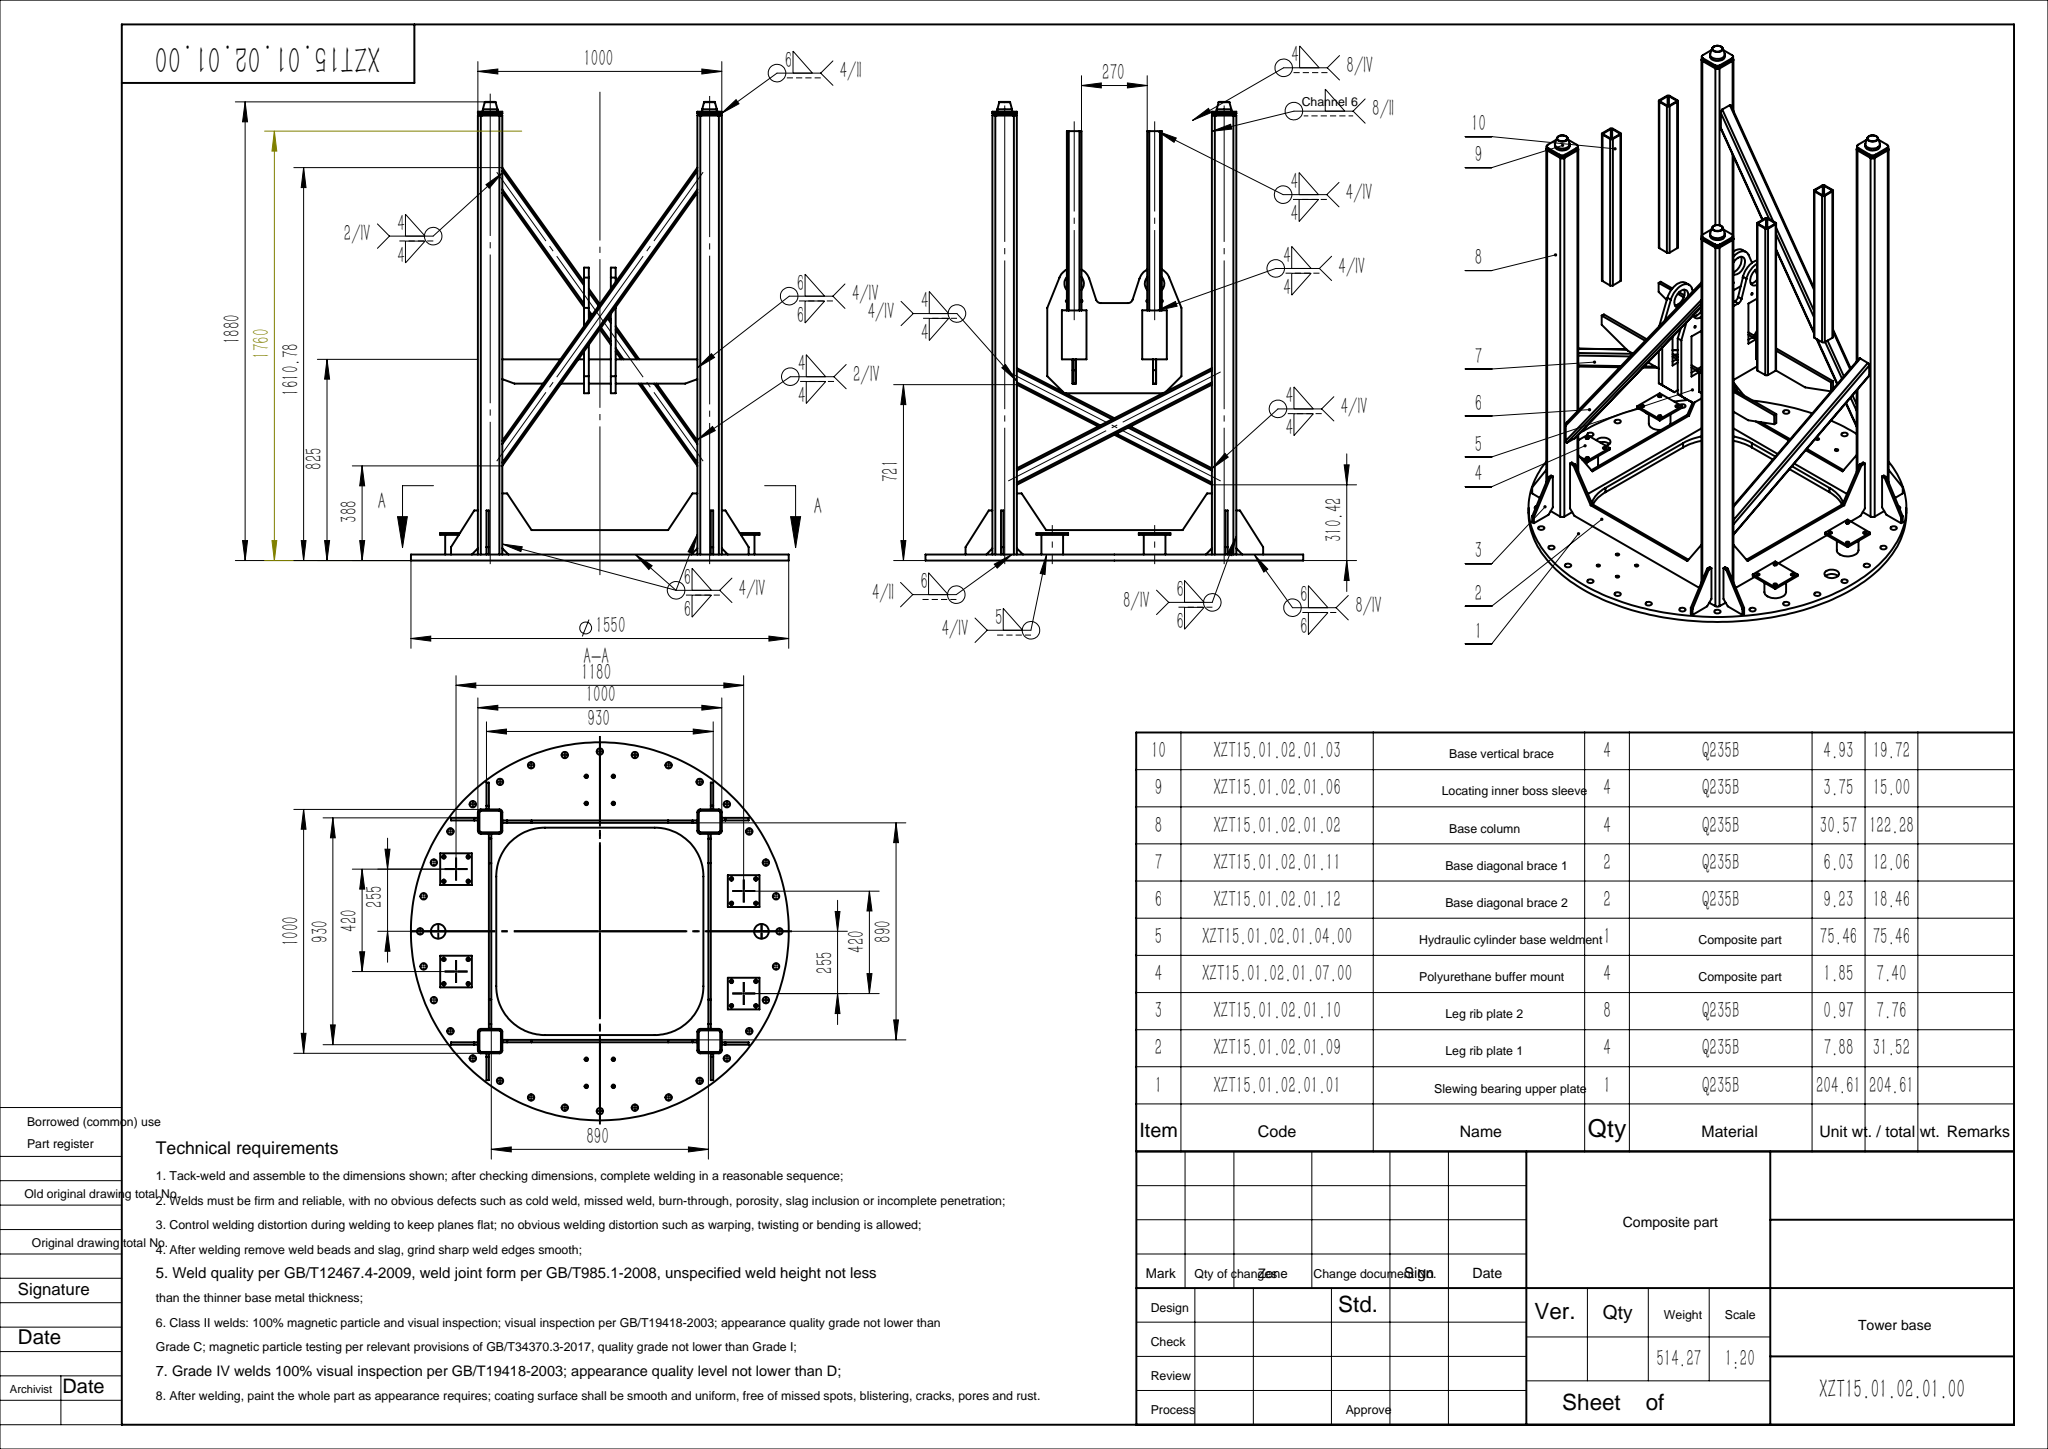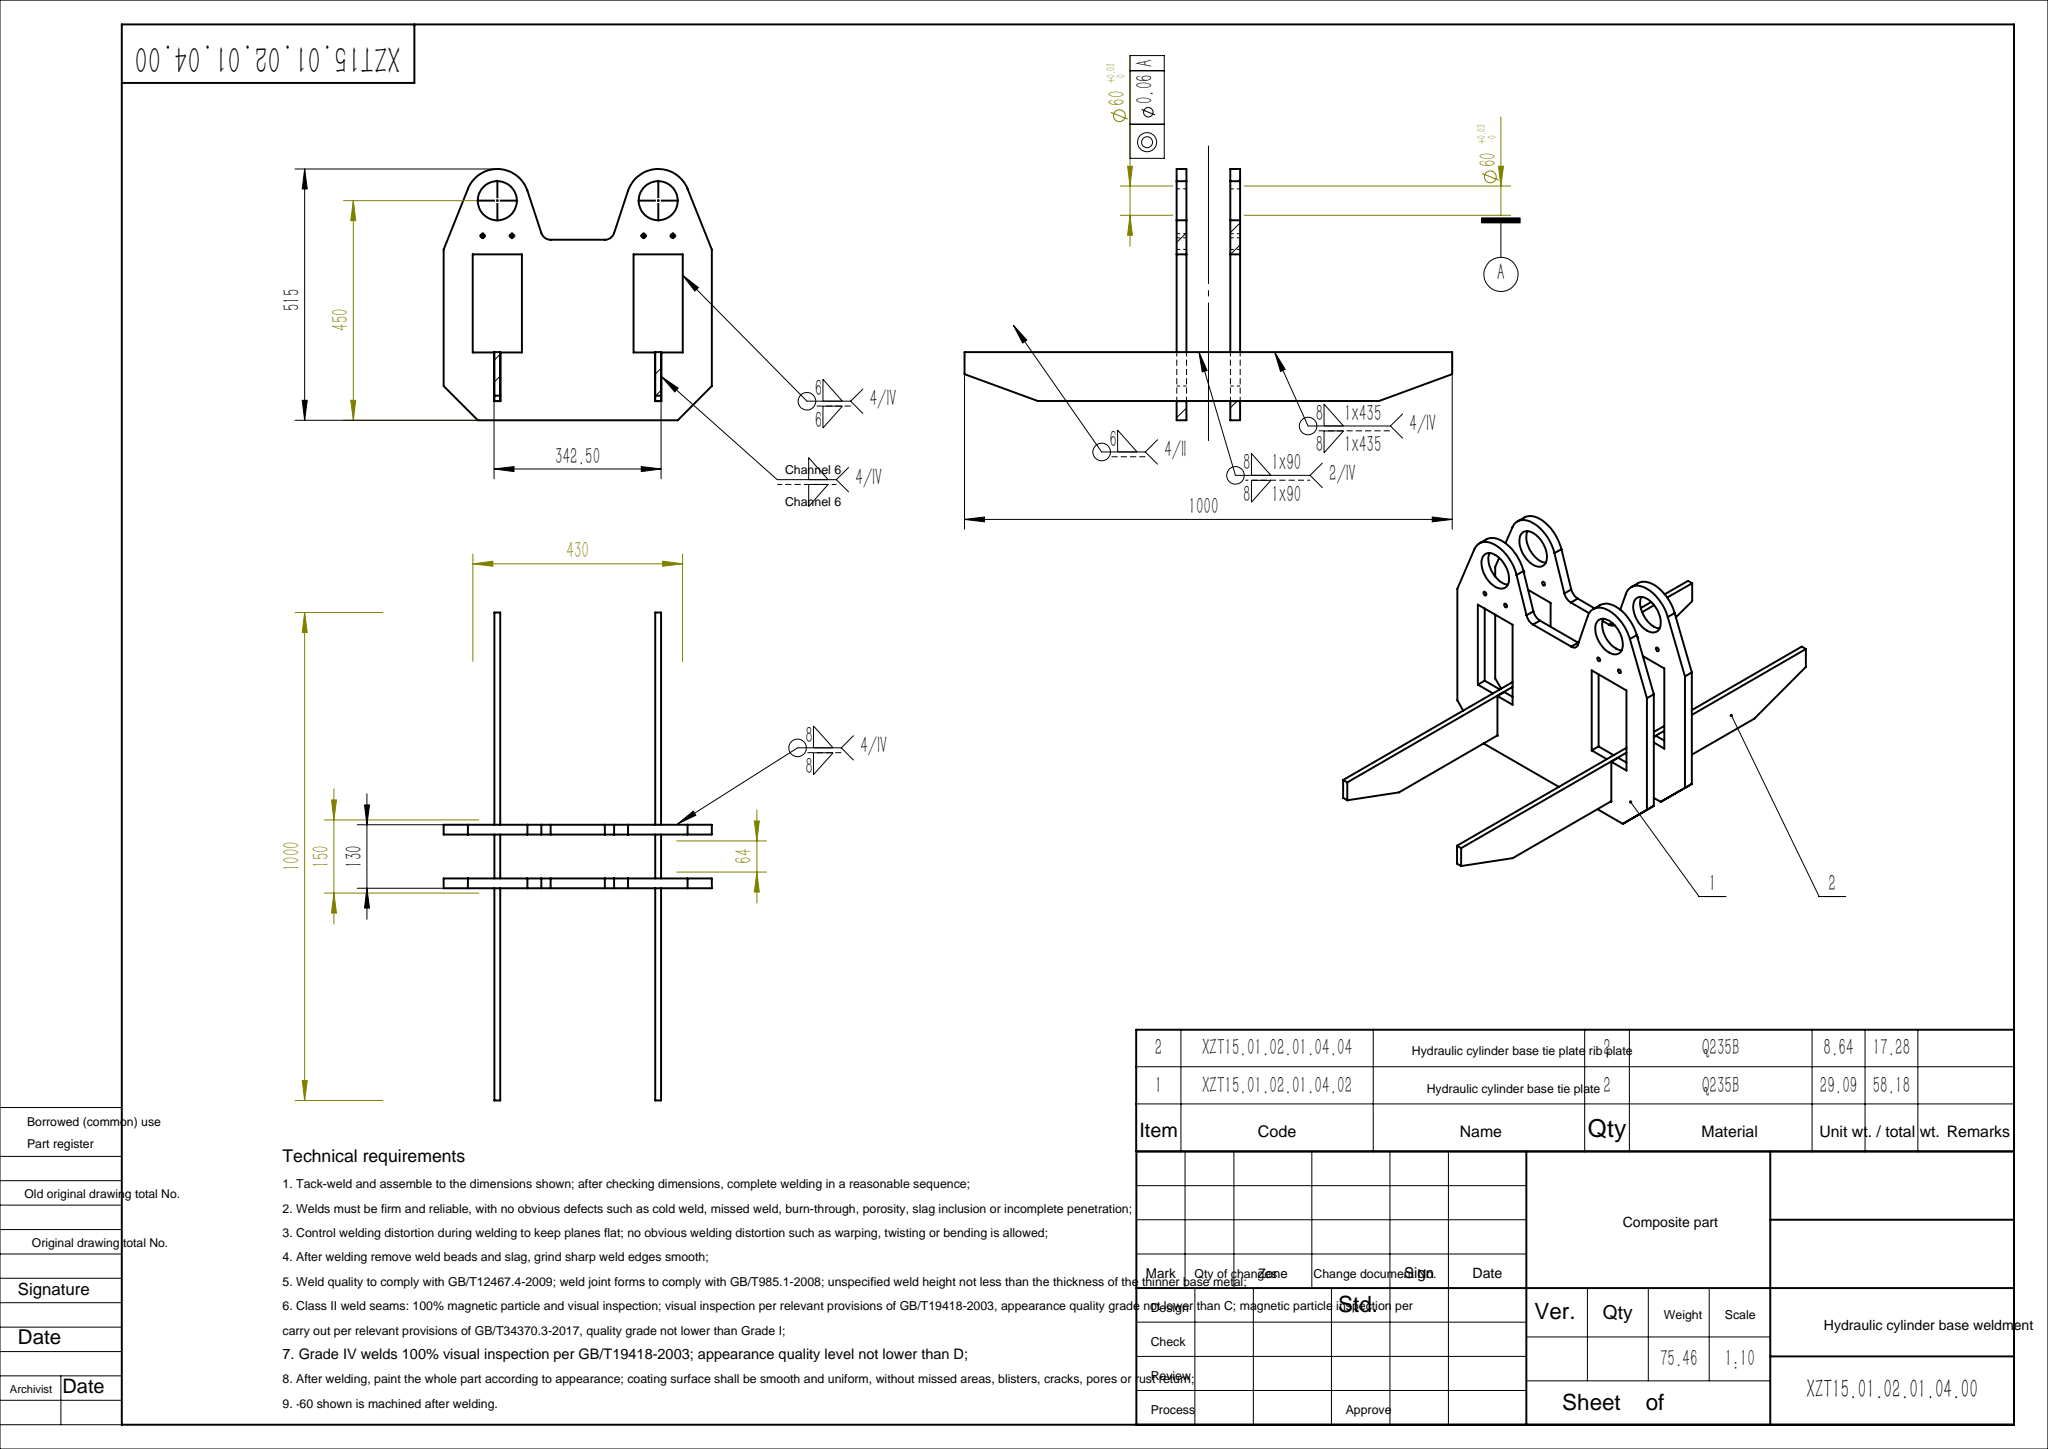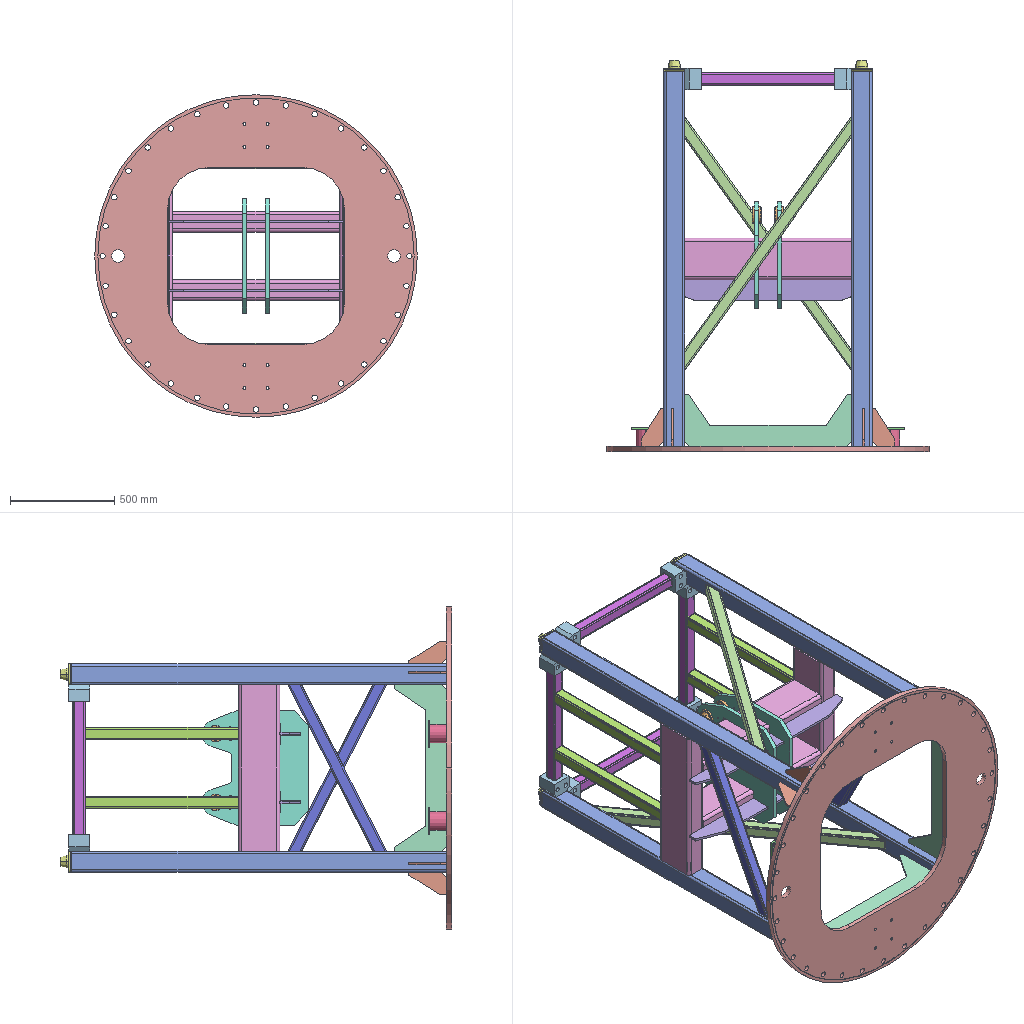Assembly | SolidWorks | 18 different items | 66 placed | box 1550 x 1880 x 1550 mm
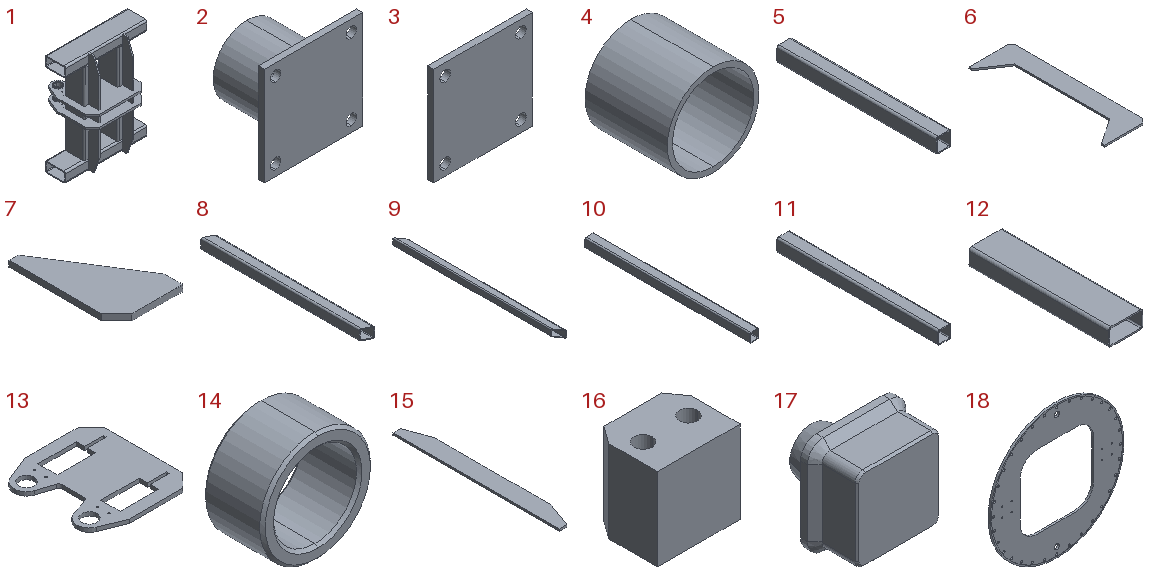Parts list (item | name | quantity | parent item | size | volume | features):
1 | (subassembly) | x1 | - | 800 x 515 x 1000 mm | 23997719 mm3 | features ReferencePattern 5, MirrorCompFeat 2
2 | (subassembly) | x4 | - | 130 x 88 x 130 mm | 235831 mm3 | -
3 | - | x4 | in 2 | 130 x 8 x 130 mm | 130274 mm3 | features Chamfer 1, Extrusion 1, Fillet 1, HoleWzd 1
4 | - | x4 | in 2 | 89 x 80 x 89 mm | 105558 mm3 | features Extrusion 1
5 | - | x4 | - | 60 x 640 x 60 mm | 547070 mm3 | features WeldMemberFeat 1, WeldmentFeature 1
6 | - | x4 | - | 250 x 800 x 10 mm | 1003750 mm3 | features Chamfer 1, Extrusion 1
7 | - | x8 | - | 110 x 180 x 10 mm | 123625 mm3 | features Chamfer 1, Extrusion 1
8 | - | x2 | - | 60 x 930 x 60 mm | 768639 mm3 | features ICE 1, WeldMemberFeat 1, WeldmentFeature 1
9 | - | x2 | - | 60 x 1460 x 60 mm | 1176227 mm3 | features ICE 1, WeldMemberFeat 1, WeldmentFeature 1
10 | - | x4 | - | 100 x 1800 x 100 mm | 3893926 mm3 | features WeldMemberFeat 1, WeldmentFeature 1
11 | - | x4 | - | 60 x 735 x 60 mm | 628275 mm3 | features WeldMemberFeat 1, WeldmentFeature 1
12 | - | x4 | in 1 | 200 x 800 x 100 mm | 3503349 mm3 | features WeldMemberFeat 1, WeldmentFeature 1
13 | - | x2 | in 1 | 515 x 550 x 20 mm | 3705557 mm3 | features Chamfer 1, Extrusion 1, Fillet 1, HoleWzd 1
14 | - | x4 | in 1 | 80 x 43 x 80 mm | 92803 mm3 | features Chamfer 1, Extrusion 1
15 | - | x2 | in 1 | 100 x 1000 x 12 mm | 1101000 mm3 | features Extrusion 1
16 | - | x8 | - | 100 x 80 x 100 mm | 692473 mm3 | features Chamfer 1, Extrusion 1, HoleWzd 1, ICE 1
17 | - | x4 | - | 100 x 90 x 100 mm | 477978 mm3 | features Chamfer 3, ICE 2, Revolution 1
18 | - | x1 | - | 1550 x 25 x 1550 mm | 26064350 mm3 | features Extrusion 1, HoleWzd 1, ICE 1
Mates (type | each side: item.copy, entity, surface, feature):
In the top assembly
Coincident | 18.1 plane | assembly plane | 3 times
Coincident | 18.1 face plane Boss-Extrude1 | 10.1 face plane GB/T 6728-2002 square hollow section 100×100×6(1)
Coincident | 18.1 face plane Boss-Extrude1 | 4.1 face plane Boss-Extrude1
Coincident | 18.1 face plane Boss-Extrude1 | 7.1 face plane Boss-Extrude1
Coincident | 10.1 face plane GB/T 6728-2002 square hollow section 100×100×6(1) | 7.1 face plane Boss-Extrude1
Coincident | 7.1 face plane Boss-Extrude1 | 7.2 face plane Boss-Extrude1
Coincident | 10.1 face plane GB/T 6728-2002 square hollow section 100×100×6(1) | 7.2 face plane Boss-Extrude1
DistanceDim | 17.1 face plane Boss-Extrude1 | 10.1 face plane GB/T 6728-2002 square hollow section 100×100×6(1)
Coincident | 10.1 face plane GB/T 6728-2002 square hollow section 100×100×6(1) | 17.1 face plane Boss-Extrude1 | 2 times
Coincident | 16.1 face plane Boss-Extrude1 | 16.2 face plane Boss-Extrude1
Coincident | 10.1 face plane GB/T 6728-2002 square hollow section 100×100×6(1) | 16.1 face plane Boss-Extrude1 | 2 times
Coincident | 16.1 face plane Boss-Extrude1 | 17.1 face plane Boss-Extrude1
Coincident | 10.1 face plane GB/T 6728-2002 square hollow section 100×100×6(1) | 16.2 face plane Boss-Extrude1 | 2 times
DistanceDim | 10.2 face plane GB/T 6728-2002 square hollow section 100×100×6(1) | 10.1 face plane GB/T 6728-2002 square hollow section 100×100×6(1)
DistanceDim | 10.1 face plane GB/T 6728-2002 square hollow section 100×100×6(1) | 10.3 face plane GB/T 6728-2002 square hollow section 100×100×6(1)
Coincident | 10.1 face plane GB/T 6728-2002 square hollow section 100×100×6(1) | 12.1 face plane GB/T 6728-2002 rectangular hollow section 200X100X8(2) | 2 times
DistanceDim | 18.1 face plane Boss-Extrude1 | 12.1 face plane GB/T 6728-2002 rectangular hollow section 200X100X8(2)
Coincident | 5.1 face plane GB/T 6728-2002 square hollow section 60×60×4(1) | 5.2 face plane GB/T 6728-2002 square hollow section 60×60×4(1)
Coincident | 16.1 face plane Boss-Extrude1 | 5.1 face plane GB/T 6728-2002 square hollow section 60×60×4(1)
Coincident | 16.2 face plane Boss-Extrude1 | 5.2 face plane GB/T 6728-2002 square hollow section 60×60×4(1)
Width | 5.1 face plane GB/T 6728-2002 square hollow section 60×60×4(1) | 5.1 face plane GB/T 6728-2002 square hollow section 60×60×4(1) | 16.1 face plane Boss-Extrude1 | 16.1 face plane Boss-Extrude1 | 2 times
Width | 5.2 face plane GB/T 6728-2002 square hollow section 60×60×4(1) | 5.2 face plane GB/T 6728-2002 square hollow section 60×60×4(1) | 16.2 face plane Boss-Extrude1 | 16.2 face plane Boss-Extrude1
Coincident | 9.1 face plane Cut-Extrude1 | 10.2 face plane GB/T 6728-2002 square hollow section 100×100×6(1)
Width | 9.1 face plane GB/T 6728-2002 square hollow section 60×60×4(1) | 9.1 face plane GB/T 6728-2002 square hollow section 60×60×4(1) | 10.2 face plane GB/T 6728-2002 square hollow section 100×100×6(1) | 10.2 face plane GB/T 6728-2002 square hollow section 100×100×6(1)
Coincident | 10.1 face plane GB/T 6728-2002 square hollow section 100×100×6(1) | 8.1 face plane Cut-Extrude1
Width | 10.1 face plane GB/T 6728-2002 square hollow section 100×100×6(1) | 10.1 face plane GB/T 6728-2002 square hollow section 100×100×6(1) | 8.1 face plane GB/T 6728-2002 square hollow section 60×60×4(1) | 8.1 face plane GB/T 6728-2002 square hollow section 60×60×4(1)
DistanceDim | 18.1 face plane Boss-Extrude1 | 8.1 edge
DistanceDim | 2.1 plane | assembly plane | 2 times
DistanceDim | 9.1 edge | 18.1 face plane Boss-Extrude1
Coincident | 18.1 face plane Boss-Extrude1 | 6.1 face plane Boss-Extrude1
Width | 6.1 face plane Boss-Extrude1 | 6.1 face plane Boss-Extrude1 | 10.1 face plane GB/T 6728-2002 square hollow section 100×100×6(1) | 10.1 face plane GB/T 6728-2002 square hollow section 100×100×6(1)
Coincident | 10.1 face plane GB/T 6728-2002 square hollow section 100×100×6(1) | 6.1 face plane Boss-Extrude1
Coincident | 18.1 face plane Boss-Extrude1 | 6.2 face plane Boss-Extrude1
Coincident | 10.1 face plane GB/T 6728-2002 square hollow section 100×100×6(1) | 6.2 face plane Boss-Extrude1
Width | 6.2 face plane Boss-Extrude1 | 6.2 face plane Boss-Extrude1 | 10.1 face plane GB/T 6728-2002 square hollow section 100×100×6(1) | 10.1 face plane GB/T 6728-2002 square hollow section 100×100×6(1)
Coincident | 11.1 face plane GB/T 6728-2002 square hollow section 60×60×4(1) | 12.1 face plane GB/T 6728-2002 rectangular hollow section 200X100X8(2)
Coincident | 11.1 face plane GB/T 6728-2002 square hollow section 60×60×4(1) | 5.2 face plane GB/T 6728-2002 square hollow section 60×60×4(1)
DistanceDim | 11.2 face plane GB/T 6728-2002 square hollow section 60×60×4(1) | 11.1 face plane GB/T 6728-2002 square hollow section 60×60×4(1)
DistanceDim | 7.1 face plane Boss-Extrude1 | 10.1 face plane GB/T 6728-2002 square hollow section 100×100×6(1)
DistanceDim | 7.2 face plane Boss-Extrude1 | 10.1 face plane GB/T 6728-2002 square hollow section 100×100×6(1)
In subassembly 2
Coordinate | 4.2 select_type:25 | 2.2 select_type:11
Coincident | 3.1 face plane Boss-Extrude1 | 4.2 face plane Boss-Extrude1
Coincident | 3.1 plane | 2.2 plane | 2 times
In subassembly 1
Coincident | 12.2 face plane GB/T 6728-2002 rectangular hollow section 200X100X8(2) | 1.1 plane
Coincident | 12.2 face plane GB/T 6728-2002 rectangular hollow section 200X100X8(2) | 12.3 face plane GB/T 6728-2002 rectangular hollow section 200X100X8(2) | 2 times
Symmetric | 12.2 face plane GB/T 6728-2002 rectangular hollow section 200X100X8(2) | 12.3 face plane GB/T 6728-2002 rectangular hollow section 200X100X8(2) | 1.1 plane
Symmetric | 12.4 face plane GB/T 6728-2002 rectangular hollow section 200X100X8(2) | 12.5 face plane GB/T 6728-2002 rectangular hollow section 200X100X8(2) | 1.1 plane
Coincident | 12.2 face plane GB/T 6728-2002 rectangular hollow section 200X100X8(2) | 12.5 face plane GB/T 6728-2002 rectangular hollow section 200X100X8(2)
Coincident | 12.3 face plane GB/T 6728-2002 rectangular hollow section 200X100X8(2) | 12.5 face plane GB/T 6728-2002 rectangular hollow section 200X100X8(2)
Coincident | 12.4 face plane GB/T 6728-2002 rectangular hollow section 200X100X8(2) | 12.5 face plane GB/T 6728-2002 rectangular hollow section 200X100X8(2) | 2 times
DistanceDim | 12.5 face plane GB/T 6728-2002 rectangular hollow section 200X100X8(2) | 12.4 face plane GB/T 6728-2002 rectangular hollow section 200X100X8(2)
Symmetric | 12.3 face plane GB/T 6728-2002 rectangular hollow section 200X100X8(2) | 12.3 face plane GB/T 6728-2002 rectangular hollow section 200X100X8(2) | 1.1 plane
Width | 13.1 face plane Boss-Extrude1 | 13.1 face plane Boss-Extrude1 | 12.5 face plane GB/T 6728-2002 rectangular hollow section 200X100X8(2) | 12.5 face plane GB/T 6728-2002 rectangular hollow section 200X100X8(2) | 2 times
Coincident | 12.2 face plane GB/T 6728-2002 rectangular hollow section 200X100X8(2) | 12.4 face plane GB/T 6728-2002 rectangular hollow section 200X100X8(2)
DistanceDim | 13.1 face plane Boss-Extrude1 | 13.2 face plane Boss-Extrude1
Coincident | 12.4 face plane GB/T 6728-2002 rectangular hollow section 200X100X8(2) | 15.1 face plane Boss-Extrude1
Coincident | 12.3 face plane GB/T 6728-2002 rectangular hollow section 200X100X8(2) | 15.1 face plane Boss-Extrude1
Width | 15.1 face plane Boss-Extrude1 | 15.1 face plane Boss-Extrude1 | 12.4 face plane GB/T 6728-2002 rectangular hollow section 200X100X8(2) | 12.4 face plane GB/T 6728-2002 rectangular hollow section 200X100X8(2)
Concentric | 14.1 face cylinder Boss-Extrude1 | 13.2 face cylinder Boss-Extrude1
DistanceDim | 14.2 face plane Boss-Extrude1 | 14.1 face plane Boss-Extrude1